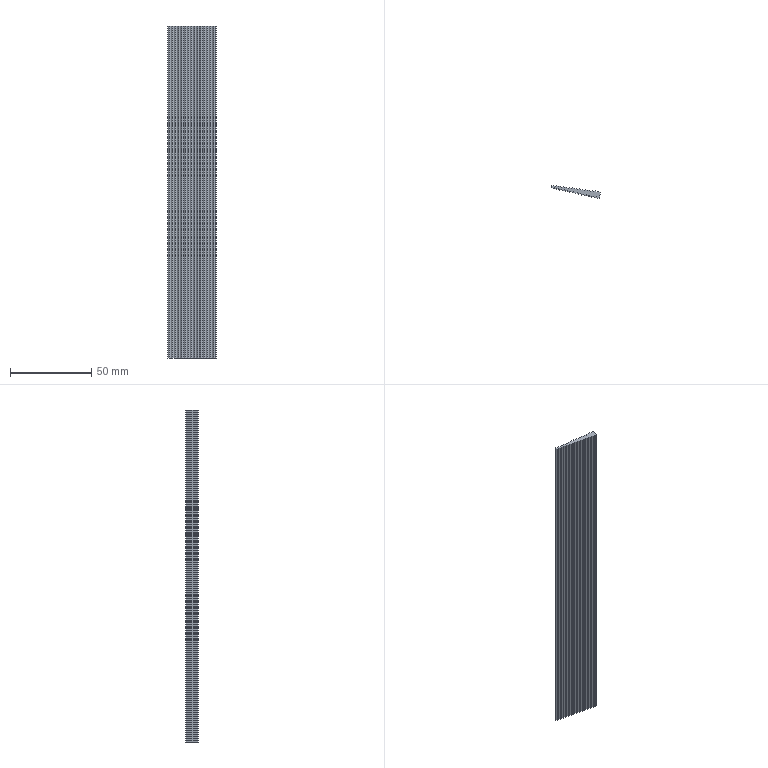Part | SolidWorks | features BaseBody 1 | 1 solid | 64 faces | box 29.865 x 7.735 x 204 mm | volume 15088 mm3 | plane 62 | cylinder 2 | commonest cylinder face diameters 16 x1 76 x1